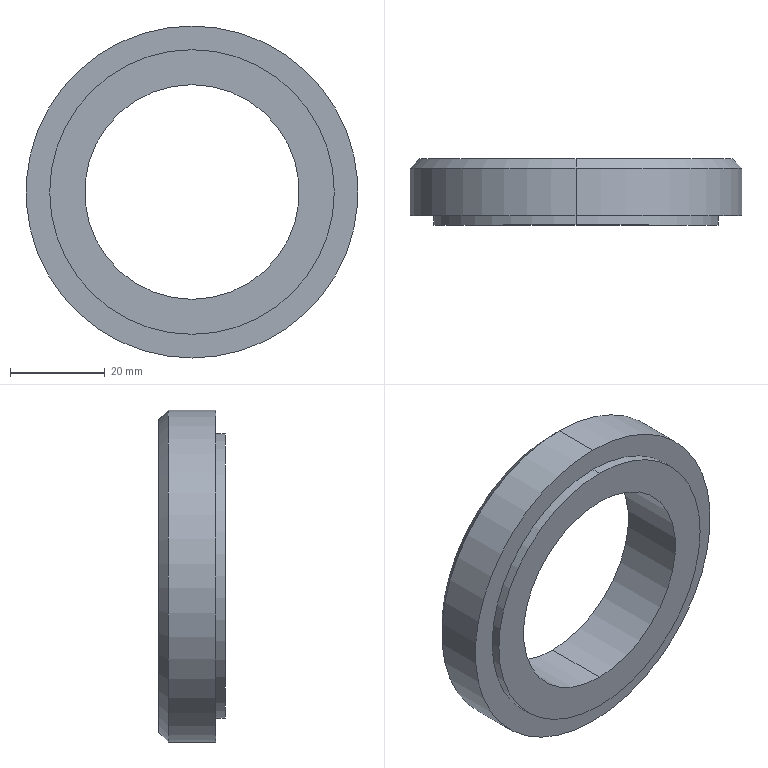Part | SolidWorks | features HoleWzd 1, Revolution 1 | 1 solid | 11 faces | box 70 x 14 x 70 mm | volume 28891 mm3 | cylinder 6 | plane 3 | cone 2 | commonest cylinder face diameters 45.25 x2 60 x2 70 x2
STEP:
#1=CARTESIAN_POINT('',(0.,0.,22.625));
#2=VERTEX_POINT('',#1);
#3=CARTESIAN_POINT('',(0.,0.,-22.625));
#4=VERTEX_POINT('',#3);
#5=CARTESIAN_POINT('',(0.,0.,0.));
#6=DIRECTION('',(0.,-1.,0.));
#7=DIRECTION('',(0.,0.,-1.));
#8=AXIS2_PLACEMENT_3D('',#5,#6,#7);
#9=CIRCLE('',#8,22.625);
#10=EDGE_CURVE('',#2,#4,#9,.T.);
#11=ORIENTED_EDGE('',*,*,#10,.T.);
#12=CARTESIAN_POINT('',(0.,14.,-22.625));
#13=VERTEX_POINT('',#12);
#14=CARTESIAN_POINT('',(0.,14.,-22.625));
#15=DIRECTION('',(0.,1.,0.));
#16=VECTOR('',#15,1000.);
#17=LINE('',#14,#16);
#18=EDGE_CURVE('',#4,#13,#17,.T.);
#19=ORIENTED_EDGE('',*,*,#18,.T.);
#20=CARTESIAN_POINT('',(0.,14.,22.625));
#21=VERTEX_POINT('',#20);
#22=CARTESIAN_POINT('',(0.,14.,0.));
#23=DIRECTION('',(0.,1.,0.));
#24=DIRECTION('',(0.,0.,1.));
#25=AXIS2_PLACEMENT_3D('',#22,#23,#24);
#26=CIRCLE('',#25,22.625);
#27=EDGE_CURVE('',#13,#21,#26,.T.);
#28=ORIENTED_EDGE('',*,*,#27,.T.);
#29=CARTESIAN_POINT('',(0.,14.,22.625));
#30=DIRECTION('',(0.,1.,0.));
#31=VECTOR('',#30,1000.);
#32=LINE('',#29,#31);
#33=EDGE_CURVE('',#2,#21,#32,.T.);
#34=ORIENTED_EDGE('',*,*,#33,.F.);
#35=EDGE_LOOP('',(#11,#19,#28,#34));
#36=FACE_OUTER_BOUND('',#35,.T.);
#37=CARTESIAN_POINT('',(0.,14.,0.));
#38=DIRECTION('',(0.,1.,0.));
#39=DIRECTION('',(0.,0.,1.));
#40=AXIS2_PLACEMENT_3D('',#37,#38,#39);
#41=CYLINDRICAL_SURFACE('',#40,22.625);
#42=ADVANCED_FACE('',(#36),#41,.F.);
#43=CARTESIAN_POINT('',(0.,14.,-33.));
#44=VERTEX_POINT('',#43);
#45=CARTESIAN_POINT('',(0.,14.,33.));
#46=VERTEX_POINT('',#45);
#47=CARTESIAN_POINT('',(0.,14.,0.));
#48=DIRECTION('',(0.,-1.,0.));
#49=DIRECTION('',(0.,0.,-1.));
#50=AXIS2_PLACEMENT_3D('',#47,#48,#49);
#51=CIRCLE('',#50,33.);
#52=EDGE_CURVE('',#44,#46,#51,.T.);
#53=ORIENTED_EDGE('',*,*,#52,.T.);
#54=CARTESIAN_POINT('',(0.,12.,35.));
#55=VERTEX_POINT('',#54);
#56=CARTESIAN_POINT('',(0.,12.,35.));
#57=DIRECTION('',(0.,-0.7071,0.7071));
#58=VECTOR('',#57,1000.);
#59=LINE('',#56,#58);
#60=EDGE_CURVE('',#46,#55,#59,.T.);
#61=ORIENTED_EDGE('',*,*,#60,.T.);
#62=CARTESIAN_POINT('',(0.,12.,-35.));
#63=VERTEX_POINT('',#62);
#64=CARTESIAN_POINT('',(0.,12.,0.));
#65=DIRECTION('',(0.,-1.,0.));
#66=DIRECTION('',(0.,0.,-1.));
#67=AXIS2_PLACEMENT_3D('',#64,#65,#66);
#68=CIRCLE('',#67,35.);
#69=EDGE_CURVE('',#63,#55,#68,.T.);
#70=ORIENTED_EDGE('',*,*,#69,.F.);
#71=CARTESIAN_POINT('',(0.,12.,-35.));
#72=DIRECTION('',(0.,-0.7071,-0.7071));
#73=VECTOR('',#72,1000.);
#74=LINE('',#71,#73);
#75=EDGE_CURVE('',#44,#63,#74,.T.);
#76=ORIENTED_EDGE('',*,*,#75,.F.);
#77=EDGE_LOOP('',(#53,#61,#70,#76));
#78=FACE_OUTER_BOUND('',#77,.T.);
#79=CARTESIAN_POINT('',(0.,12.,0.));
#80=DIRECTION('',(0.,-1.,0.));
#81=DIRECTION('',(0.,0.,-1.));
#82=AXIS2_PLACEMENT_3D('',#79,#80,#81);
#83=CONICAL_SURFACE('',#82,35.,0.7854);
#84=ADVANCED_FACE('',(#78),#83,.T.);
#85=ORIENTED_EDGE('',*,*,#69,.T.);
#86=CARTESIAN_POINT('',(0.,2.,35.));
#87=VERTEX_POINT('',#86);
#88=CARTESIAN_POINT('',(0.,0.,35.));
#89=DIRECTION('',(0.,-1.,0.));
#90=VECTOR('',#89,1000.);
#91=LINE('',#88,#90);
#92=EDGE_CURVE('',#55,#87,#91,.T.);
#93=ORIENTED_EDGE('',*,*,#92,.T.);
#94=CARTESIAN_POINT('',(0.,2.,-35.));
#95=VERTEX_POINT('',#94);
#96=CARTESIAN_POINT('',(0.,2.,0.));
#97=DIRECTION('',(0.,-1.,0.));
#98=DIRECTION('',(0.,0.,-1.));
#99=AXIS2_PLACEMENT_3D('',#96,#97,#98);
#100=CIRCLE('',#99,35.);
#101=EDGE_CURVE('',#95,#87,#100,.T.);
#102=ORIENTED_EDGE('',*,*,#101,.F.);
#103=CARTESIAN_POINT('',(0.,0.,-35.));
#104=DIRECTION('',(0.,-1.,0.));
#105=VECTOR('',#104,1000.);
#106=LINE('',#103,#105);
#107=EDGE_CURVE('',#63,#95,#106,.T.);
#108=ORIENTED_EDGE('',*,*,#107,.F.);
#109=EDGE_LOOP('',(#85,#93,#102,#108));
#110=FACE_OUTER_BOUND('',#109,.T.);
#111=CARTESIAN_POINT('',(0.,0.,0.));
#112=DIRECTION('',(0.,-1.,0.));
#113=DIRECTION('',(0.,0.,-1.));
#114=AXIS2_PLACEMENT_3D('',#111,#112,#113);
#115=CYLINDRICAL_SURFACE('',#114,35.);
#116=ADVANCED_FACE('',(#110),#115,.T.);
#117=CARTESIAN_POINT('',(0.,2.,-30.));
#118=VERTEX_POINT('',#117);
#119=CARTESIAN_POINT('',(0.,2.,30.));
#120=VERTEX_POINT('',#119);
#121=CARTESIAN_POINT('',(0.,2.,0.));
#122=DIRECTION('',(0.,-1.,0.));
#123=DIRECTION('',(0.,0.,-1.));
#124=AXIS2_PLACEMENT_3D('',#121,#122,#123);
#125=CIRCLE('',#124,30.);
#126=EDGE_CURVE('',#118,#120,#125,.T.);
#127=ORIENTED_EDGE('',*,*,#126,.T.);
#128=CARTESIAN_POINT('',(0.,0.,30.));
#129=VERTEX_POINT('',#128);
#130=CARTESIAN_POINT('',(0.,0.,30.));
#131=DIRECTION('',(0.,-1.,0.));
#132=VECTOR('',#131,1000.);
#133=LINE('',#130,#132);
#134=EDGE_CURVE('',#120,#129,#133,.T.);
#135=ORIENTED_EDGE('',*,*,#134,.T.);
#136=CARTESIAN_POINT('',(0.,0.,-30.));
#137=VERTEX_POINT('',#136);
#138=CARTESIAN_POINT('',(0.,0.,0.));
#139=DIRECTION('',(0.,-1.,0.));
#140=DIRECTION('',(0.,0.,-1.));
#141=AXIS2_PLACEMENT_3D('',#138,#139,#140);
#142=CIRCLE('',#141,30.);
#143=EDGE_CURVE('',#137,#129,#142,.T.);
#144=ORIENTED_EDGE('',*,*,#143,.F.);
#145=CARTESIAN_POINT('',(0.,0.,-30.));
#146=DIRECTION('',(0.,-1.,0.));
#147=VECTOR('',#146,1000.);
#148=LINE('',#145,#147);
#149=EDGE_CURVE('',#118,#137,#148,.T.);
#150=ORIENTED_EDGE('',*,*,#149,.F.);
#151=EDGE_LOOP('',(#127,#135,#144,#150));
#152=FACE_OUTER_BOUND('',#151,.T.);
#153=CARTESIAN_POINT('',(0.,0.,0.));
#154=DIRECTION('',(0.,-1.,0.));
#155=DIRECTION('',(0.,0.,-1.));
#156=AXIS2_PLACEMENT_3D('',#153,#154,#155);
#157=CYLINDRICAL_SURFACE('',#156,30.);
#158=ADVANCED_FACE('',(#152),#157,.T.);
#159=ORIENTED_EDGE('',*,*,#10,.F.);
#160=CARTESIAN_POINT('',(0.,0.,0.));
#161=DIRECTION('',(0.,-1.,0.));
#162=DIRECTION('',(0.,0.,-1.));
#163=AXIS2_PLACEMENT_3D('',#160,#161,#162);
#164=CIRCLE('',#163,22.625);
#165=EDGE_CURVE('',#4,#2,#164,.T.);
#166=ORIENTED_EDGE('',*,*,#165,.F.);
#167=EDGE_LOOP('',(#159,#166));
#168=FACE_BOUND('',#167,.T.);
#169=ORIENTED_EDGE('',*,*,#143,.T.);
#170=CARTESIAN_POINT('',(0.,0.,0.));
#171=DIRECTION('',(0.,-1.,0.));
#172=DIRECTION('',(0.,0.,-1.));
#173=AXIS2_PLACEMENT_3D('',#170,#171,#172);
#174=CIRCLE('',#173,30.);
#175=EDGE_CURVE('',#129,#137,#174,.T.);
#176=ORIENTED_EDGE('',*,*,#175,.T.);
#177=EDGE_LOOP('',(#169,#176));
#178=FACE_OUTER_BOUND('',#177,.T.);
#179=CARTESIAN_POINT('',(0.,0.,-22.5));
#180=DIRECTION('',(0.,-1.,0.));
#181=DIRECTION('',(0.,0.,-1.));
#182=AXIS2_PLACEMENT_3D('',#179,#180,#181);
#183=PLANE('',#182);
#184=ADVANCED_FACE('',(#168,#178),#183,.T.);
#185=ORIENTED_EDGE('',*,*,#134,.F.);
#186=CARTESIAN_POINT('',(0.,2.,0.));
#187=DIRECTION('',(0.,-1.,0.));
#188=DIRECTION('',(0.,0.,-1.));
#189=AXIS2_PLACEMENT_3D('',#186,#187,#188);
#190=CIRCLE('',#189,30.);
#191=EDGE_CURVE('',#120,#118,#190,.T.);
#192=ORIENTED_EDGE('',*,*,#191,.T.);
#193=ORIENTED_EDGE('',*,*,#149,.T.);
#194=ORIENTED_EDGE('',*,*,#175,.F.);
#195=EDGE_LOOP('',(#185,#192,#193,#194));
#196=FACE_OUTER_BOUND('',#195,.T.);
#197=CARTESIAN_POINT('',(0.,0.,0.));
#198=DIRECTION('',(0.,-1.,0.));
#199=DIRECTION('',(0.,0.,-1.));
#200=AXIS2_PLACEMENT_3D('',#197,#198,#199);
#201=CYLINDRICAL_SURFACE('',#200,30.);
#202=ADVANCED_FACE('',(#196),#201,.T.);
#203=ORIENTED_EDGE('',*,*,#101,.T.);
#204=CARTESIAN_POINT('',(0.,2.,0.));
#205=DIRECTION('',(0.,-1.,0.));
#206=DIRECTION('',(0.,0.,-1.));
#207=AXIS2_PLACEMENT_3D('',#204,#205,#206);
#208=CIRCLE('',#207,35.);
#209=EDGE_CURVE('',#87,#95,#208,.T.);
#210=ORIENTED_EDGE('',*,*,#209,.T.);
#211=EDGE_LOOP('',(#203,#210));
#212=FACE_OUTER_BOUND('',#211,.T.);
#213=ORIENTED_EDGE('',*,*,#126,.F.);
#214=ORIENTED_EDGE('',*,*,#191,.F.);
#215=EDGE_LOOP('',(#213,#214));
#216=FACE_BOUND('',#215,.T.);
#217=CARTESIAN_POINT('',(0.,2.,-30.));
#218=DIRECTION('',(0.,-1.,0.));
#219=DIRECTION('',(0.,0.,-1.));
#220=AXIS2_PLACEMENT_3D('',#217,#218,#219);
#221=PLANE('',#220);
#222=ADVANCED_FACE('',(#212,#216),#221,.T.);
#223=ORIENTED_EDGE('',*,*,#92,.F.);
#224=CARTESIAN_POINT('',(0.,12.,0.));
#225=DIRECTION('',(0.,-1.,0.));
#226=DIRECTION('',(0.,0.,-1.));
#227=AXIS2_PLACEMENT_3D('',#224,#225,#226);
#228=CIRCLE('',#227,35.);
#229=EDGE_CURVE('',#55,#63,#228,.T.);
#230=ORIENTED_EDGE('',*,*,#229,.T.);
#231=ORIENTED_EDGE('',*,*,#107,.T.);
#232=ORIENTED_EDGE('',*,*,#209,.F.);
#233=EDGE_LOOP('',(#223,#230,#231,#232));
#234=FACE_OUTER_BOUND('',#233,.T.);
#235=CARTESIAN_POINT('',(0.,0.,0.));
#236=DIRECTION('',(0.,-1.,0.));
#237=DIRECTION('',(0.,0.,-1.));
#238=AXIS2_PLACEMENT_3D('',#235,#236,#237);
#239=CYLINDRICAL_SURFACE('',#238,35.);
#240=ADVANCED_FACE('',(#234),#239,.T.);
#241=ORIENTED_EDGE('',*,*,#60,.F.);
#242=CARTESIAN_POINT('',(0.,14.,0.));
#243=DIRECTION('',(0.,-1.,0.));
#244=DIRECTION('',(0.,0.,-1.));
#245=AXIS2_PLACEMENT_3D('',#242,#243,#244);
#246=CIRCLE('',#245,33.);
#247=EDGE_CURVE('',#46,#44,#246,.T.);
#248=ORIENTED_EDGE('',*,*,#247,.T.);
#249=ORIENTED_EDGE('',*,*,#75,.T.);
#250=ORIENTED_EDGE('',*,*,#229,.F.);
#251=EDGE_LOOP('',(#241,#248,#249,#250));
#252=FACE_OUTER_BOUND('',#251,.T.);
#253=CARTESIAN_POINT('',(0.,12.,0.));
#254=DIRECTION('',(0.,-1.,0.));
#255=DIRECTION('',(0.,0.,-1.));
#256=AXIS2_PLACEMENT_3D('',#253,#254,#255);
#257=CONICAL_SURFACE('',#256,35.,0.7854);
#258=ADVANCED_FACE('',(#252),#257,.T.);
#259=CARTESIAN_POINT('',(0.,14.,0.));
#260=DIRECTION('',(0.,1.,0.));
#261=DIRECTION('',(0.,0.,1.));
#262=AXIS2_PLACEMENT_3D('',#259,#260,#261);
#263=CIRCLE('',#262,22.625);
#264=EDGE_CURVE('',#21,#13,#263,.T.);
#265=ORIENTED_EDGE('',*,*,#264,.F.);
#266=ORIENTED_EDGE('',*,*,#27,.F.);
#267=EDGE_LOOP('',(#265,#266));
#268=FACE_BOUND('',#267,.T.);
#269=ORIENTED_EDGE('',*,*,#52,.F.);
#270=ORIENTED_EDGE('',*,*,#247,.F.);
#271=EDGE_LOOP('',(#269,#270));
#272=FACE_OUTER_BOUND('',#271,.T.);
#273=CARTESIAN_POINT('',(0.,14.,-33.));
#274=DIRECTION('',(0.,1.,0.));
#275=DIRECTION('',(0.,0.,1.));
#276=AXIS2_PLACEMENT_3D('',#273,#274,#275);
#277=PLANE('',#276);
#278=ADVANCED_FACE('',(#268,#272),#277,.T.);
#279=ORIENTED_EDGE('',*,*,#18,.F.);
#280=ORIENTED_EDGE('',*,*,#165,.T.);
#281=ORIENTED_EDGE('',*,*,#33,.T.);
#282=ORIENTED_EDGE('',*,*,#264,.T.);
#283=EDGE_LOOP('',(#279,#280,#281,#282));
#284=FACE_OUTER_BOUND('',#283,.T.);
#285=CARTESIAN_POINT('',(0.,14.,0.));
#286=DIRECTION('',(0.,1.,0.));
#287=DIRECTION('',(0.,0.,1.));
#288=AXIS2_PLACEMENT_3D('',#285,#286,#287);
#289=CYLINDRICAL_SURFACE('',#288,22.625);
#290=ADVANCED_FACE('',(#284),#289,.F.);
#291=CLOSED_SHELL('',(#42,#84,#116,#158,#184,#202,#222,#240,#258,#278,#290));
#292=MANIFOLD_SOLID_BREP('',#291);
#293=CARTESIAN_POINT('',(0.,0.,0.));
#294=DIRECTION('',(0.,0.,1.));
#295=DIRECTION('',(1.,0.,0.));
#296=AXIS2_PLACEMENT_3D('',#293,#294,#295);
#297=(LENGTH_UNIT()NAMED_UNIT(*)SI_UNIT(.MILLI.,.METRE.));
#298=UNCERTAINTY_MEASURE_WITH_UNIT(LENGTH_MEASURE(0.00001),#297,'','');
#299=(NAMED_UNIT(*)PLANE_ANGLE_UNIT()SI_UNIT($,.RADIAN.));
#300=(NAMED_UNIT(*)SI_UNIT($,.STERADIAN.)SOLID_ANGLE_UNIT());
#301=(GEOMETRIC_REPRESENTATION_CONTEXT(3)GLOBAL_UNCERTAINTY_ASSIGNED_CONTEXT((#298))GLOBAL_UNIT_ASSIGNED_CONTEXT((#297,#299,#300))REPRESENTATION_CONTEXT('',''));
#302=ADVANCED_BREP_SHAPE_REPRESENTATION('',(#292,#296),#301);